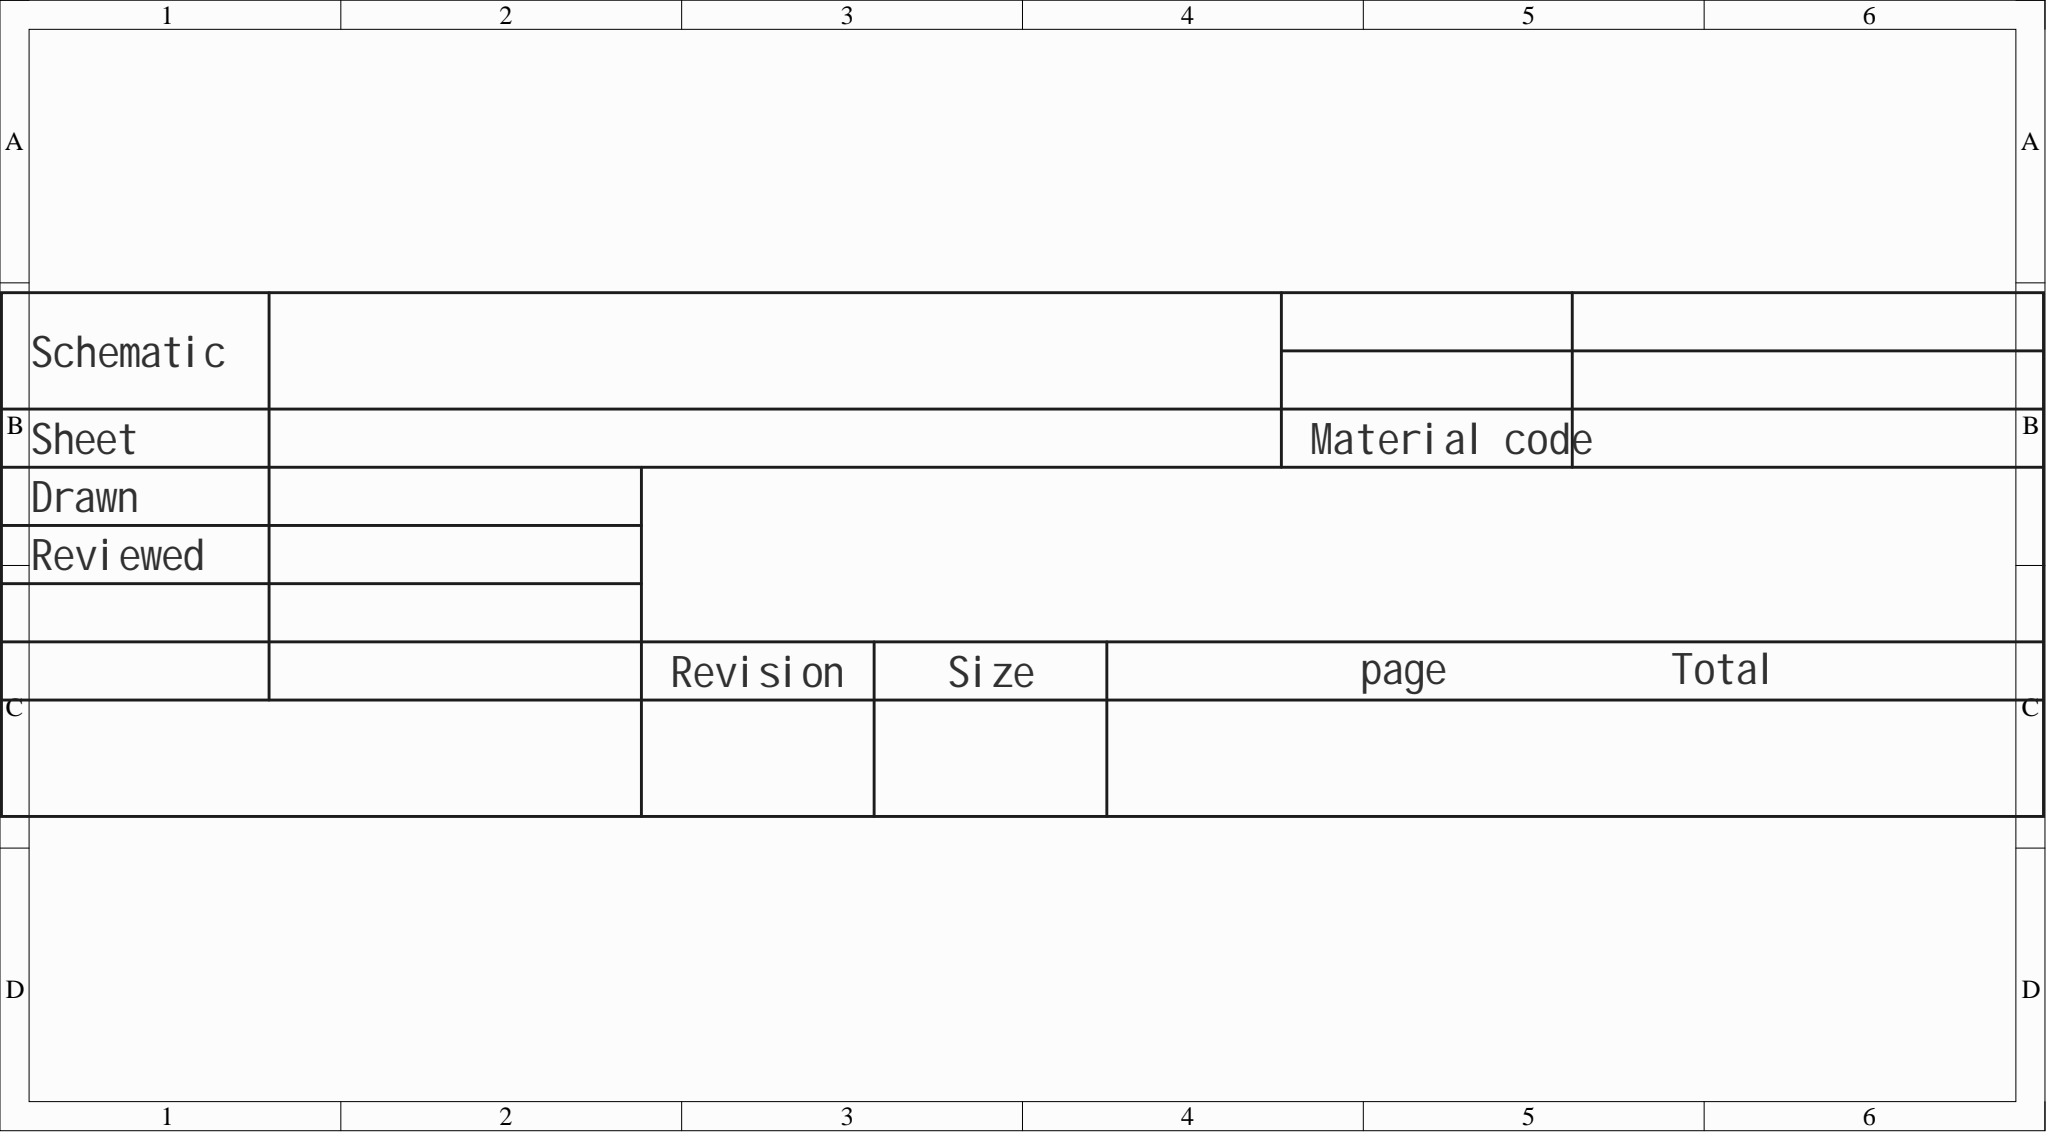Circuit board | Altium Designer | 22 parts | 29 nets
Bill of materials:
Comment,Description,Designator,Footprint,LibRef,Quantity
"10uF","Capacitance: 10uF; tolerance: ±20%; rated voltage: 50V; ripple current: 120mA@100KHz; equivalent series resistance (ESR): 1.6Ω;","C1","CAP-TH_BD5.0-P2.00-D0.8-FD-10UF50VC110GL","10UF50VC110GL","1"
"30pF","Capacitance: 30pF; tolerance: ±10%; rated voltage: 25V; temperature coefficient: C0G;","C2, C3","CAP-TH_L3.8-W2.5-P2.54-D0.50","C315C300K3G5TA7301","2"
"","","H1","HDR-TH_9P-P2.54-V-F-1","HDR-F_2.54_1x9P","1"
"","","H2","HDR-TH_4P-P2.54-V-M","HDR-M_2.54_1x4P","1"
"","","H5","HDR-TH_2P-P2.54-V-M-1","HDR-M_2.54_1x2P","1"
"LMB162ADC","16x2 character LCD module","LCD1","LCD1602","LMB162ADC","1"
"","","LED2","LED_TH-3mm","LED_TH-G_3mm","1"
"","","Q1","S8050_SOT-23","S8050_SOT_NPN","1"
"10kΩ","","R1, R4","Res_1/8W","Res_AXIAL-1/8W","2"
"10kΩ","Resistance: 10kΩ; tolerance: ±25%; power: 100mW;","R2","RES-ADJ-SMD_RM065-V1","RM065-103(10K)","1"
"220Ω","","R6","Res_1/8W","Res_AXIAL-1/8W","1"
"Tact switch 3*6*2.5","","SW1","SW-SMD_L6.0-W3.6-LS8.0","轻触按键3*6*2.5","1"
"","","SW2, SW3, SW4","Key_TH_3.5x6x4.3","Key_TH_3.5x6x4.3","3"
"STC89C516RD+40I-PDIP40","CPU core: 51 series; program storage capacity: 61KB; RAM total capacity: 1.25KB; GPIO port count: 35; operating voltage range: 3.5V~5.5V; CPU max frequency: -; program memory type: FLASH;","U1","DIP-40_L52.3-W13.9-P2.54-LS15.2-BL","STC89C516RD+40I-PDIP40","1"
"11.059MHz","Frequency: 12MHz; normal temperature frequency tolerance: ±30ppm; external load capacitance: -; frequency stability (full temperature): ±50ppm;","U2","HC-49US_L11.0-W4.6-P4.88","ECS-120-S-4","1"
"ADC0832CCN","","U3","DIP-8_L9.7-W6.4-P2.54-LS7.6-BL","ADC0832CCN","1"
"光敏电阻-5MM","","U4","RES-TH_L4.9-W4.3-P3.4","光敏电阻-5MM","1"
"100nF","","U5","CAP-TH_L5.0-W2.5-P5.00-D1.0","100nF","1"
Netlist (Protel format):
[
C1
CAP-TH_BD5.0-P2.00-D0.8-FD-10UF50VC110GL
10uF



]
[
C2
CAP-TH_L3.8-W2.5-P2.54-D0.50
30pF



]
[
C3
CAP-TH_L3.8-W2.5-P2.54-D0.50
30pF



]
[
H1
HDR-TH_9P-P2.54-V-F-1




]
[
H2
HDR-TH_4P-P2.54-V-M




]
[
H5
HDR-TH_2P-P2.54-V-M-1




]
[
LCD1
LCD1602
LMB162ADC



]
[
LED2
LED_TH-3mm




]
[
Q1
S8050_SOT-23




]
[
R1
Res_1/8W
10kΩ



]
[
R2
RES-ADJ-SMD_RM065-V1
10kΩ



]
[
R4
Res_1/8W
10kΩ



]
[
R6
Res_1/8W
220Ω



]
[
SW1
SW-SMD_L6.0-W3.6-LS8.0
Tact switch 3*6*2.5



]
[
SW2
Key_TH_3.5x6x4.3




]
[
SW3
Key_TH_3.5x6x4.3




]
[
SW4
Key_TH_3.5x6x4.3




]
[
U1
DIP-40_L52.3-W13.9-P2.54-LS15.2-BL
STC89C516RD+40I-PDIP40



]
[
U2
HC-49US_L11.0-W4.6-P4.88
11.0592MHz



]
[
U3
DIP-8_L9.7-W6.4-P2.54-LS7.6-BL
ADC0832CCN



]
[
U4
RES-TH_L4.9-W4.3-P3.4
光敏电阻-5MM



]
[
U5
CAP-TH_L5.0-W2.5-P5.00-D1.0
100nF



]
(
VCC
C1-1
H1-1
H2-1
H5-2
LCD1-2
LCD1-15
R2-1
R6-2
SW1-2
U1-40
U3-8
U4-1
U5-1
)
(
TXD
H2-3
U1-11
)
(
RXD
H2-2
U1-10
)
(
PWM
Q1-1
U1-25
)
(
NetU1_4
U1-4
U3-6
)
(
NetU1_3
U1-3
U3-5
)
(
NetU1_2
U1-2
U3-7
)
(
NetU1_1
U1-1
U3-1
)
(
NetSW4_A
SW4-A
U1-26
)
(
NetSW3_A
SW3-A
U1-27
)
(
NetSW2_A
SW2-A
U1-28
)
(
NetR4_2
R4-2
U3-2
U4-2
)
(
NetLED2_1
LED2-1
R6-1
)
(
NetLCD1_16
LCD1-16
Q1-2
)
(
NetLCD1_3
LCD1-3
R2-2
)
(
NetH1_9
H1-9
LCD1-14
U1-32
)
(
NetH1_8
H1-8
LCD1-13
U1-33
)
(
NetH1_7
H1-7
LCD1-12
U1-34
)
(
NetH1_6
H1-6
LCD1-11
U1-35
)
(
NetH1_5
H1-5
LCD1-10
U1-36
)
(
NetH1_4
H1-4
LCD1-9
U1-37
)
(
NetH1_3
H1-3
LCD1-8
U1-38
)
(
NetH1_2
H1-2
LCD1-7
U1-39
)
(
NetC3_2
C3-2
U1-19
U2-2
)
(
NetC2_2
C2-2
U1-18
U2-1
)
(
NetC1_2
C1-2
R1-2
SW1-1
U1-9
)
(
L2
LCD1-4
U1-21
)
(
L1
LCD1-6
U1-22
)
(
GND
C2-1
C3-1
H2-4
H5-1
LCD1-1
LCD1-5
LED2-2
Q1-3
R1-1
R2-3
R4-1
SW2-B
SW3-B
SW4-B
U1-20
U3-3
U3-4
U5-2
)